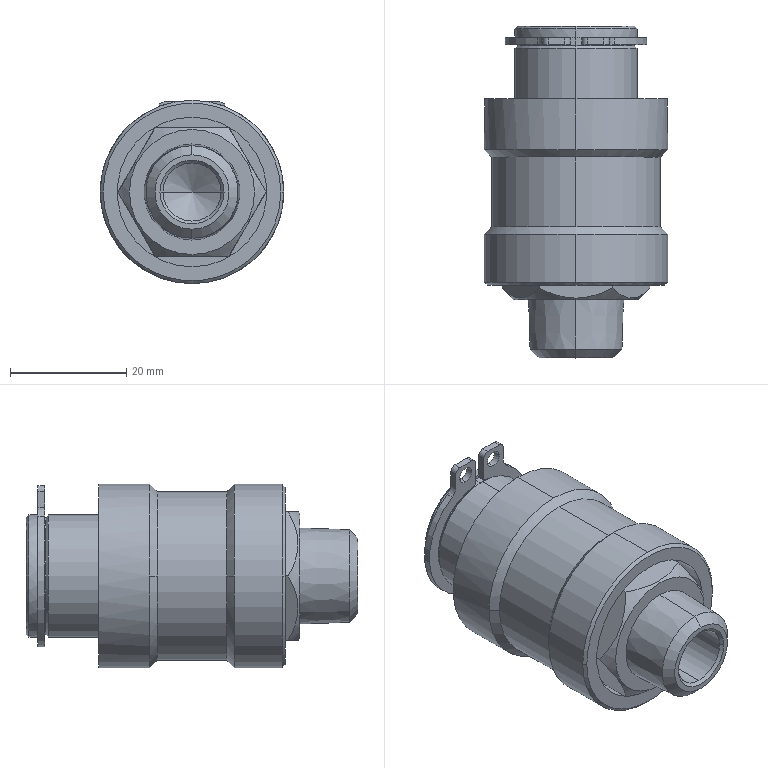Part | STEP file | MVHS-10A_default | 1 solid | 77 faces | box 31.5 x 57 x 31.5 mm | volume 23556 mm3 | cylinder 32 | plane 23 | cone 22 | commonest cylinder face diameters 1.921 x4 2.881 x4 21 x4 31.5 x4 3.842 x2 10 x2